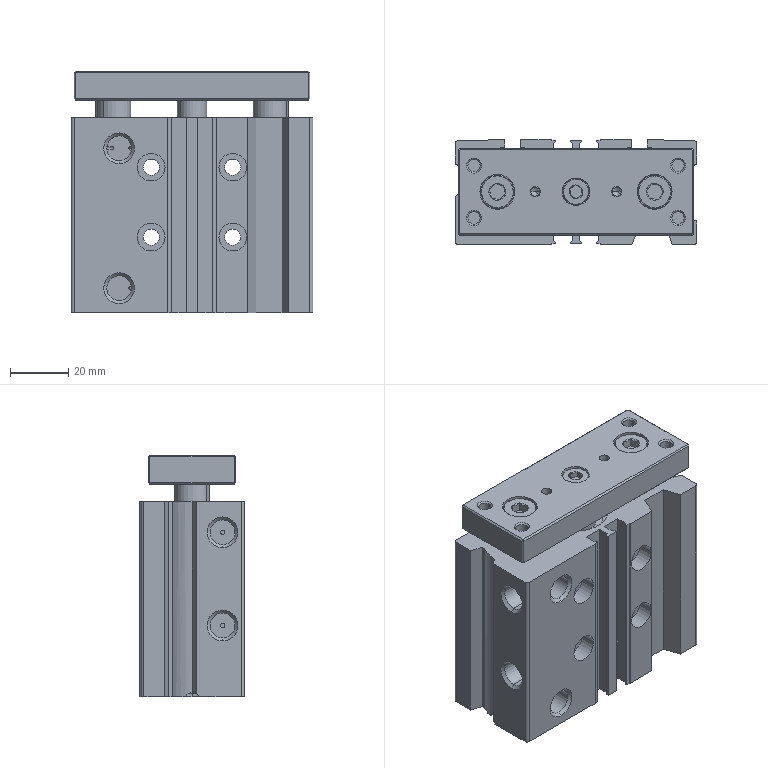Part | 13 solids | 548 faces | box 83 x 36 x 83 mm | volume 177953 mm3 | cylinder 233 | plane 197 | cone 103 | torus 12 | spline 3 | commonest cylinder face diameters 5 x45 4.2 x18 1.5 x16 3 x12 3.5 x12 8 x12